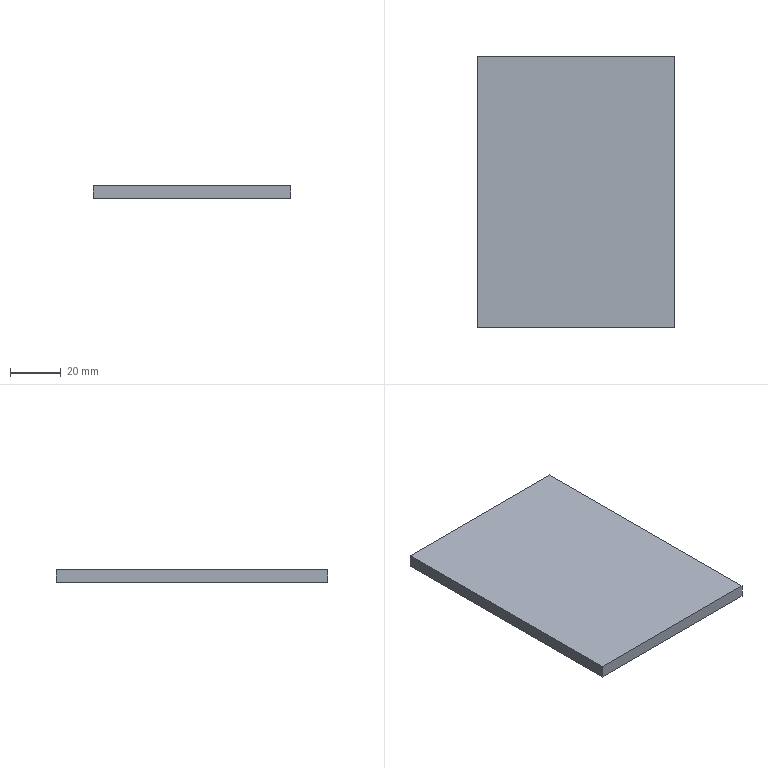Part | STEP file | Guide wheel mechanism revised.sldasm-Part-499 | 1 solid | 6 faces | box 78 x 107 x 5 mm | volume 41730 mm3 | plane 6
STEP:
#1=CARTESIAN_POINT('',(78.,112.,-65.5));
#2=VERTEX_POINT('',#1);
#3=CARTESIAN_POINT('',(78.,5.,-65.5));
#4=VERTEX_POINT('',#3);
#5=CARTESIAN_POINT('',(78.,112.,-65.5));
#6=DIRECTION('',(0.,-1.,0.));
#7=VECTOR('',#6,1000.);
#8=LINE('',#5,#7);
#9=EDGE_CURVE('',#2,#4,#8,.T.);
#10=ORIENTED_EDGE('',*,*,#9,.F.);
#11=CARTESIAN_POINT('',(78.,112.,-60.5));
#12=VERTEX_POINT('',#11);
#13=CARTESIAN_POINT('',(78.,112.,-60.5));
#14=DIRECTION('',(0.,0.,-1.));
#15=VECTOR('',#14,1000.);
#16=LINE('',#13,#15);
#17=EDGE_CURVE('',#12,#2,#16,.T.);
#18=ORIENTED_EDGE('',*,*,#17,.F.);
#19=CARTESIAN_POINT('',(78.,5.,-60.5));
#20=VERTEX_POINT('',#19);
#21=CARTESIAN_POINT('',(78.,112.,-60.5));
#22=DIRECTION('',(0.,-1.,0.));
#23=VECTOR('',#22,1000.);
#24=LINE('',#21,#23);
#25=EDGE_CURVE('',#12,#20,#24,.T.);
#26=ORIENTED_EDGE('',*,*,#25,.T.);
#27=CARTESIAN_POINT('',(78.,5.,-60.5));
#28=DIRECTION('',(0.,0.,-1.));
#29=VECTOR('',#28,1000.);
#30=LINE('',#27,#29);
#31=EDGE_CURVE('',#20,#4,#30,.T.);
#32=ORIENTED_EDGE('',*,*,#31,.T.);
#33=EDGE_LOOP('',(#10,#18,#26,#32));
#34=FACE_OUTER_BOUND('',#33,.T.);
#35=CARTESIAN_POINT('',(78.,112.,-60.5));
#36=DIRECTION('',(1.,0.,0.));
#37=DIRECTION('',(0.,0.,-1.));
#38=AXIS2_PLACEMENT_3D('',#35,#36,#37);
#39=PLANE('',#38);
#40=ADVANCED_FACE('',(#34),#39,.T.);
#41=CARTESIAN_POINT('',(0.,112.,-65.5));
#42=VERTEX_POINT('',#41);
#43=CARTESIAN_POINT('',(78.,112.,-65.5));
#44=DIRECTION('',(1.,0.,0.));
#45=VECTOR('',#44,1000.);
#46=LINE('',#43,#45);
#47=EDGE_CURVE('',#42,#2,#46,.T.);
#48=ORIENTED_EDGE('',*,*,#47,.F.);
#49=CARTESIAN_POINT('',(0.,112.,-60.5));
#50=VERTEX_POINT('',#49);
#51=CARTESIAN_POINT('',(0.,112.,-60.5));
#52=DIRECTION('',(0.,0.,-1.));
#53=VECTOR('',#52,1000.);
#54=LINE('',#51,#53);
#55=EDGE_CURVE('',#50,#42,#54,.T.);
#56=ORIENTED_EDGE('',*,*,#55,.F.);
#57=CARTESIAN_POINT('',(78.,112.,-60.5));
#58=DIRECTION('',(1.,0.,0.));
#59=VECTOR('',#58,1000.);
#60=LINE('',#57,#59);
#61=EDGE_CURVE('',#50,#12,#60,.T.);
#62=ORIENTED_EDGE('',*,*,#61,.T.);
#63=ORIENTED_EDGE('',*,*,#17,.T.);
#64=EDGE_LOOP('',(#48,#56,#62,#63));
#65=FACE_OUTER_BOUND('',#64,.T.);
#66=CARTESIAN_POINT('',(78.,112.,-60.5));
#67=DIRECTION('',(0.,1.,0.));
#68=DIRECTION('',(0.,0.,1.));
#69=AXIS2_PLACEMENT_3D('',#66,#67,#68);
#70=PLANE('',#69);
#71=ADVANCED_FACE('',(#65),#70,.T.);
#72=CARTESIAN_POINT('',(0.,5.,-65.5));
#73=VERTEX_POINT('',#72);
#74=CARTESIAN_POINT('',(0.,112.,-65.5));
#75=DIRECTION('',(0.,1.,0.));
#76=VECTOR('',#75,1000.);
#77=LINE('',#74,#76);
#78=EDGE_CURVE('',#73,#42,#77,.T.);
#79=ORIENTED_EDGE('',*,*,#78,.F.);
#80=CARTESIAN_POINT('',(0.,5.,-60.5));
#81=VERTEX_POINT('',#80);
#82=CARTESIAN_POINT('',(0.,5.,-60.5));
#83=DIRECTION('',(0.,0.,-1.));
#84=VECTOR('',#83,1000.);
#85=LINE('',#82,#84);
#86=EDGE_CURVE('',#81,#73,#85,.T.);
#87=ORIENTED_EDGE('',*,*,#86,.F.);
#88=CARTESIAN_POINT('',(0.,112.,-60.5));
#89=DIRECTION('',(0.,1.,0.));
#90=VECTOR('',#89,1000.);
#91=LINE('',#88,#90);
#92=EDGE_CURVE('',#81,#50,#91,.T.);
#93=ORIENTED_EDGE('',*,*,#92,.T.);
#94=ORIENTED_EDGE('',*,*,#55,.T.);
#95=EDGE_LOOP('',(#79,#87,#93,#94));
#96=FACE_OUTER_BOUND('',#95,.T.);
#97=CARTESIAN_POINT('',(0.,112.,-60.5));
#98=DIRECTION('',(-1.,0.,0.));
#99=DIRECTION('',(0.,0.,1.));
#100=AXIS2_PLACEMENT_3D('',#97,#98,#99);
#101=PLANE('',#100);
#102=ADVANCED_FACE('',(#96),#101,.T.);
#103=CARTESIAN_POINT('',(78.,5.,-65.5));
#104=DIRECTION('',(-1.,0.,0.));
#105=VECTOR('',#104,1000.);
#106=LINE('',#103,#105);
#107=EDGE_CURVE('',#4,#73,#106,.T.);
#108=ORIENTED_EDGE('',*,*,#107,.F.);
#109=ORIENTED_EDGE('',*,*,#31,.F.);
#110=CARTESIAN_POINT('',(78.,5.,-60.5));
#111=DIRECTION('',(-1.,0.,0.));
#112=VECTOR('',#111,1000.);
#113=LINE('',#110,#112);
#114=EDGE_CURVE('',#20,#81,#113,.T.);
#115=ORIENTED_EDGE('',*,*,#114,.T.);
#116=ORIENTED_EDGE('',*,*,#86,.T.);
#117=EDGE_LOOP('',(#108,#109,#115,#116));
#118=FACE_OUTER_BOUND('',#117,.T.);
#119=CARTESIAN_POINT('',(78.,5.,-60.5));
#120=DIRECTION('',(0.,-1.,0.));
#121=DIRECTION('',(0.,0.,-1.));
#122=AXIS2_PLACEMENT_3D('',#119,#120,#121);
#123=PLANE('',#122);
#124=ADVANCED_FACE('',(#118),#123,.T.);
#125=ORIENTED_EDGE('',*,*,#25,.F.);
#126=ORIENTED_EDGE('',*,*,#61,.F.);
#127=ORIENTED_EDGE('',*,*,#92,.F.);
#128=ORIENTED_EDGE('',*,*,#114,.F.);
#129=EDGE_LOOP('',(#125,#126,#127,#128));
#130=FACE_OUTER_BOUND('',#129,.T.);
#131=CARTESIAN_POINT('',(0.,0.,-60.5));
#132=DIRECTION('',(0.,0.,-1.));
#133=DIRECTION('',(-1.,0.,0.));
#134=AXIS2_PLACEMENT_3D('',#131,#132,#133);
#135=PLANE('',#134);
#136=ADVANCED_FACE('',(#130),#135,.F.);
#137=ORIENTED_EDGE('',*,*,#9,.T.);
#138=ORIENTED_EDGE('',*,*,#107,.T.);
#139=ORIENTED_EDGE('',*,*,#78,.T.);
#140=ORIENTED_EDGE('',*,*,#47,.T.);
#141=EDGE_LOOP('',(#137,#138,#139,#140));
#142=FACE_OUTER_BOUND('',#141,.T.);
#143=CARTESIAN_POINT('',(0.,0.,-65.5));
#144=DIRECTION('',(0.,0.,-1.));
#145=DIRECTION('',(-1.,0.,0.));
#146=AXIS2_PLACEMENT_3D('',#143,#144,#145);
#147=PLANE('',#146);
#148=ADVANCED_FACE('',(#142),#147,.T.);
#149=CLOSED_SHELL('',(#40,#71,#102,#124,#136,#148));
#150=MANIFOLD_SOLID_BREP('',#149);
#151=CARTESIAN_POINT('',(0.,0.,0.));
#152=DIRECTION('',(0.,0.,1.));
#153=DIRECTION('',(1.,0.,0.));
#154=AXIS2_PLACEMENT_3D('',#151,#152,#153);
#155=(LENGTH_UNIT()NAMED_UNIT(*)SI_UNIT(.MILLI.,.METRE.));
#156=UNCERTAINTY_MEASURE_WITH_UNIT(LENGTH_MEASURE(0.00001),#155,'','');
#157=(NAMED_UNIT(*)PLANE_ANGLE_UNIT()SI_UNIT($,.RADIAN.));
#158=(NAMED_UNIT(*)SI_UNIT($,.STERADIAN.)SOLID_ANGLE_UNIT());
#159=(GEOMETRIC_REPRESENTATION_CONTEXT(3)GLOBAL_UNCERTAINTY_ASSIGNED_CONTEXT((#156))GLOBAL_UNIT_ASSIGNED_CONTEXT((#155,#157,#158))REPRESENTATION_CONTEXT('',''));
#160=ADVANCED_BREP_SHAPE_REPRESENTATION('',(#150,#154),#159);